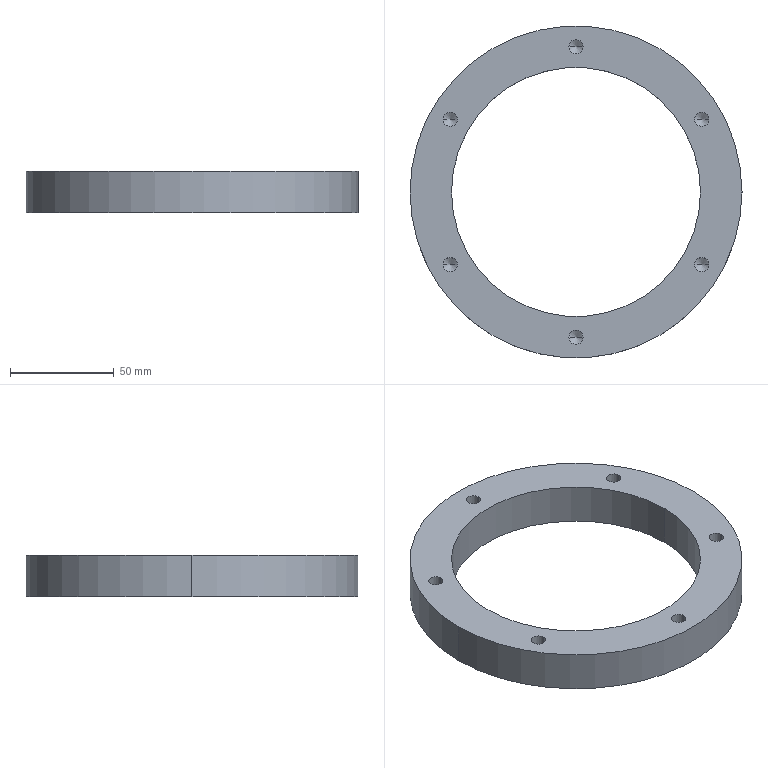Part | SolidWorks | features 3DProfileFeature 1, Extrusion 1, HoleWzd 1 | 1 solid | 30 faces | box 160 x 160 x 20 mm | volume 171859 mm3 | cylinder 16 | cone 12 | plane 2 | commonest cylinder face diameters 6.8 x12 120 x2 160 x2
STEP:
#1=CARTESIAN_POINT('',(-3.4,70.,2.));
#2=VERTEX_POINT('',#1);
#3=CARTESIAN_POINT('',(3.4,70.,2.));
#4=VERTEX_POINT('',#3);
#5=CARTESIAN_POINT('',(0.,70.,2.));
#6=DIRECTION('',(0.,0.,1.));
#7=DIRECTION('',(1.,0.,0.));
#8=AXIS2_PLACEMENT_3D('',#5,#6,#7);
#9=CIRCLE('',#8,3.4);
#10=EDGE_CURVE('',#2,#4,#9,.T.);
#11=ORIENTED_EDGE('',*,*,#10,.F.);
#12=CARTESIAN_POINT('',(-3.4,70.,20.));
#13=VERTEX_POINT('',#12);
#14=CARTESIAN_POINT('',(-3.4,70.,20.));
#15=DIRECTION('',(0.,0.,1.));
#16=VECTOR('',#15,1000.);
#17=LINE('',#14,#16);
#18=EDGE_CURVE('',#2,#13,#17,.T.);
#19=ORIENTED_EDGE('',*,*,#18,.T.);
#20=CARTESIAN_POINT('',(3.4,70.,20.));
#21=VERTEX_POINT('',#20);
#22=CARTESIAN_POINT('',(0.,70.,20.));
#23=DIRECTION('',(0.,0.,1.));
#24=DIRECTION('',(1.,0.,0.));
#25=AXIS2_PLACEMENT_3D('',#22,#23,#24);
#26=CIRCLE('',#25,3.4);
#27=EDGE_CURVE('',#13,#21,#26,.T.);
#28=ORIENTED_EDGE('',*,*,#27,.T.);
#29=CARTESIAN_POINT('',(3.4,70.,20.));
#30=DIRECTION('',(0.,0.,1.));
#31=VECTOR('',#30,1000.);
#32=LINE('',#29,#31);
#33=EDGE_CURVE('',#4,#21,#32,.T.);
#34=ORIENTED_EDGE('',*,*,#33,.F.);
#35=EDGE_LOOP('',(#11,#19,#28,#34));
#36=FACE_OUTER_BOUND('',#35,.T.);
#37=CARTESIAN_POINT('',(0.,70.,20.));
#38=DIRECTION('',(0.,0.,1.));
#39=DIRECTION('',(1.,0.,0.));
#40=AXIS2_PLACEMENT_3D('',#37,#38,#39);
#41=CYLINDRICAL_SURFACE('',#40,3.4);
#42=ADVANCED_FACE('',(#36),#41,.F.);
#43=CARTESIAN_POINT('',(-0.07144,70.,0.));
#44=VERTEX_POINT('',#43);
#45=CARTESIAN_POINT('',(0.07144,70.,0.));
#46=VERTEX_POINT('',#45);
#47=CARTESIAN_POINT('',(0.,70.,0.));
#48=DIRECTION('',(0.,0.,1.));
#49=DIRECTION('',(1.,0.,0.));
#50=AXIS2_PLACEMENT_3D('',#47,#48,#49);
#51=CIRCLE('',#50,0.07144);
#52=EDGE_CURVE('',#44,#46,#51,.T.);
#53=ORIENTED_EDGE('',*,*,#52,.F.);
#54=CARTESIAN_POINT('',(-3.4,70.,2.));
#55=DIRECTION('',(-0.8572,0.,0.515));
#56=VECTOR('',#55,1000.);
#57=LINE('',#54,#56);
#58=EDGE_CURVE('',#44,#2,#57,.T.);
#59=ORIENTED_EDGE('',*,*,#58,.T.);
#60=ORIENTED_EDGE('',*,*,#10,.T.);
#61=CARTESIAN_POINT('',(3.4,70.,2.));
#62=DIRECTION('',(0.8572,0.,0.515));
#63=VECTOR('',#62,1000.);
#64=LINE('',#61,#63);
#65=EDGE_CURVE('',#46,#4,#64,.T.);
#66=ORIENTED_EDGE('',*,*,#65,.F.);
#67=EDGE_LOOP('',(#53,#59,#60,#66));
#68=FACE_OUTER_BOUND('',#67,.T.);
#69=CARTESIAN_POINT('',(0.,70.,2.));
#70=DIRECTION('',(0.,0.,1.));
#71=DIRECTION('',(1.,0.,0.));
#72=AXIS2_PLACEMENT_3D('',#69,#70,#71);
#73=CONICAL_SURFACE('',#72,3.4,1.03);
#74=ADVANCED_FACE('',(#68),#73,.F.);
#75=CARTESIAN_POINT('',(57.222,35.,2.));
#76=VERTEX_POINT('',#75);
#77=CARTESIAN_POINT('',(64.022,35.,2.));
#78=VERTEX_POINT('',#77);
#79=CARTESIAN_POINT('',(60.622,35.,2.));
#80=DIRECTION('',(0.,0.,1.));
#81=DIRECTION('',(1.,0.,0.));
#82=AXIS2_PLACEMENT_3D('',#79,#80,#81);
#83=CIRCLE('',#82,3.4);
#84=EDGE_CURVE('',#76,#78,#83,.T.);
#85=ORIENTED_EDGE('',*,*,#84,.F.);
#86=CARTESIAN_POINT('',(57.222,35.,20.));
#87=VERTEX_POINT('',#86);
#88=CARTESIAN_POINT('',(57.222,35.,20.));
#89=DIRECTION('',(0.,0.,1.));
#90=VECTOR('',#89,1000.);
#91=LINE('',#88,#90);
#92=EDGE_CURVE('',#76,#87,#91,.T.);
#93=ORIENTED_EDGE('',*,*,#92,.T.);
#94=CARTESIAN_POINT('',(64.022,35.,20.));
#95=VERTEX_POINT('',#94);
#96=CARTESIAN_POINT('',(60.622,35.,20.));
#97=DIRECTION('',(0.,0.,1.));
#98=DIRECTION('',(1.,0.,0.));
#99=AXIS2_PLACEMENT_3D('',#96,#97,#98);
#100=CIRCLE('',#99,3.4);
#101=EDGE_CURVE('',#87,#95,#100,.T.);
#102=ORIENTED_EDGE('',*,*,#101,.T.);
#103=CARTESIAN_POINT('',(64.022,35.,20.));
#104=DIRECTION('',(0.,0.,1.));
#105=VECTOR('',#104,1000.);
#106=LINE('',#103,#105);
#107=EDGE_CURVE('',#78,#95,#106,.T.);
#108=ORIENTED_EDGE('',*,*,#107,.F.);
#109=EDGE_LOOP('',(#85,#93,#102,#108));
#110=FACE_OUTER_BOUND('',#109,.T.);
#111=CARTESIAN_POINT('',(60.622,35.,20.));
#112=DIRECTION('',(0.,0.,1.));
#113=DIRECTION('',(1.,0.,0.));
#114=AXIS2_PLACEMENT_3D('',#111,#112,#113);
#115=CYLINDRICAL_SURFACE('',#114,3.4);
#116=ADVANCED_FACE('',(#110),#115,.F.);
#117=CARTESIAN_POINT('',(60.55,35.,0.));
#118=VERTEX_POINT('',#117);
#119=CARTESIAN_POINT('',(60.693,35.,0.));
#120=VERTEX_POINT('',#119);
#121=CARTESIAN_POINT('',(60.622,35.,0.));
#122=DIRECTION('',(0.,0.,1.));
#123=DIRECTION('',(1.,0.,0.));
#124=AXIS2_PLACEMENT_3D('',#121,#122,#123);
#125=CIRCLE('',#124,0.07144);
#126=EDGE_CURVE('',#118,#120,#125,.T.);
#127=ORIENTED_EDGE('',*,*,#126,.F.);
#128=CARTESIAN_POINT('',(57.222,35.,2.));
#129=DIRECTION('',(-0.8572,0.,0.515));
#130=VECTOR('',#129,1000.);
#131=LINE('',#128,#130);
#132=EDGE_CURVE('',#118,#76,#131,.T.);
#133=ORIENTED_EDGE('',*,*,#132,.T.);
#134=ORIENTED_EDGE('',*,*,#84,.T.);
#135=CARTESIAN_POINT('',(64.022,35.,2.));
#136=DIRECTION('',(0.8572,0.,0.515));
#137=VECTOR('',#136,1000.);
#138=LINE('',#135,#137);
#139=EDGE_CURVE('',#120,#78,#138,.T.);
#140=ORIENTED_EDGE('',*,*,#139,.F.);
#141=EDGE_LOOP('',(#127,#133,#134,#140));
#142=FACE_OUTER_BOUND('',#141,.T.);
#143=CARTESIAN_POINT('',(60.622,35.,2.));
#144=DIRECTION('',(0.,0.,1.));
#145=DIRECTION('',(1.,0.,0.));
#146=AXIS2_PLACEMENT_3D('',#143,#144,#145);
#147=CONICAL_SURFACE('',#146,3.4,1.03);
#148=ADVANCED_FACE('',(#142),#147,.F.);
#149=CARTESIAN_POINT('',(57.222,-35.,2.));
#150=VERTEX_POINT('',#149);
#151=CARTESIAN_POINT('',(64.022,-35.,2.));
#152=VERTEX_POINT('',#151);
#153=CARTESIAN_POINT('',(60.622,-35.,2.));
#154=DIRECTION('',(0.,0.,1.));
#155=DIRECTION('',(1.,0.,0.));
#156=AXIS2_PLACEMENT_3D('',#153,#154,#155);
#157=CIRCLE('',#156,3.4);
#158=EDGE_CURVE('',#150,#152,#157,.T.);
#159=ORIENTED_EDGE('',*,*,#158,.F.);
#160=CARTESIAN_POINT('',(57.222,-35.,20.));
#161=VERTEX_POINT('',#160);
#162=CARTESIAN_POINT('',(57.222,-35.,20.));
#163=DIRECTION('',(0.,0.,1.));
#164=VECTOR('',#163,1000.);
#165=LINE('',#162,#164);
#166=EDGE_CURVE('',#150,#161,#165,.T.);
#167=ORIENTED_EDGE('',*,*,#166,.T.);
#168=CARTESIAN_POINT('',(64.022,-35.,20.));
#169=VERTEX_POINT('',#168);
#170=CARTESIAN_POINT('',(60.622,-35.,20.));
#171=DIRECTION('',(0.,0.,1.));
#172=DIRECTION('',(1.,0.,0.));
#173=AXIS2_PLACEMENT_3D('',#170,#171,#172);
#174=CIRCLE('',#173,3.4);
#175=EDGE_CURVE('',#161,#169,#174,.T.);
#176=ORIENTED_EDGE('',*,*,#175,.T.);
#177=CARTESIAN_POINT('',(64.022,-35.,20.));
#178=DIRECTION('',(0.,0.,1.));
#179=VECTOR('',#178,1000.);
#180=LINE('',#177,#179);
#181=EDGE_CURVE('',#152,#169,#180,.T.);
#182=ORIENTED_EDGE('',*,*,#181,.F.);
#183=EDGE_LOOP('',(#159,#167,#176,#182));
#184=FACE_OUTER_BOUND('',#183,.T.);
#185=CARTESIAN_POINT('',(60.622,-35.,20.));
#186=DIRECTION('',(0.,0.,1.));
#187=DIRECTION('',(1.,0.,0.));
#188=AXIS2_PLACEMENT_3D('',#185,#186,#187);
#189=CYLINDRICAL_SURFACE('',#188,3.4);
#190=ADVANCED_FACE('',(#184),#189,.F.);
#191=CARTESIAN_POINT('',(60.55,-35.,0.));
#192=VERTEX_POINT('',#191);
#193=CARTESIAN_POINT('',(60.693,-35.,0.));
#194=VERTEX_POINT('',#193);
#195=CARTESIAN_POINT('',(60.622,-35.,0.));
#196=DIRECTION('',(0.,0.,1.));
#197=DIRECTION('',(1.,0.,0.));
#198=AXIS2_PLACEMENT_3D('',#195,#196,#197);
#199=CIRCLE('',#198,0.07144);
#200=EDGE_CURVE('',#192,#194,#199,.T.);
#201=ORIENTED_EDGE('',*,*,#200,.F.);
#202=CARTESIAN_POINT('',(57.222,-35.,2.));
#203=DIRECTION('',(-0.8572,0.,0.515));
#204=VECTOR('',#203,1000.);
#205=LINE('',#202,#204);
#206=EDGE_CURVE('',#192,#150,#205,.T.);
#207=ORIENTED_EDGE('',*,*,#206,.T.);
#208=ORIENTED_EDGE('',*,*,#158,.T.);
#209=CARTESIAN_POINT('',(64.022,-35.,2.));
#210=DIRECTION('',(0.8572,0.,0.515));
#211=VECTOR('',#210,1000.);
#212=LINE('',#209,#211);
#213=EDGE_CURVE('',#194,#152,#212,.T.);
#214=ORIENTED_EDGE('',*,*,#213,.F.);
#215=EDGE_LOOP('',(#201,#207,#208,#214));
#216=FACE_OUTER_BOUND('',#215,.T.);
#217=CARTESIAN_POINT('',(60.622,-35.,2.));
#218=DIRECTION('',(0.,0.,1.));
#219=DIRECTION('',(1.,0.,0.));
#220=AXIS2_PLACEMENT_3D('',#217,#218,#219);
#221=CONICAL_SURFACE('',#220,3.4,1.03);
#222=ADVANCED_FACE('',(#216),#221,.F.);
#223=CARTESIAN_POINT('',(-3.4,-70.,2.));
#224=VERTEX_POINT('',#223);
#225=CARTESIAN_POINT('',(3.4,-70.,2.));
#226=VERTEX_POINT('',#225);
#227=CARTESIAN_POINT('',(0.,-70.,2.));
#228=DIRECTION('',(0.,0.,1.));
#229=DIRECTION('',(1.,0.,0.));
#230=AXIS2_PLACEMENT_3D('',#227,#228,#229);
#231=CIRCLE('',#230,3.4);
#232=EDGE_CURVE('',#224,#226,#231,.T.);
#233=ORIENTED_EDGE('',*,*,#232,.F.);
#234=CARTESIAN_POINT('',(-3.4,-70.,20.));
#235=VERTEX_POINT('',#234);
#236=CARTESIAN_POINT('',(-3.4,-70.,20.));
#237=DIRECTION('',(0.,0.,1.));
#238=VECTOR('',#237,1000.);
#239=LINE('',#236,#238);
#240=EDGE_CURVE('',#224,#235,#239,.T.);
#241=ORIENTED_EDGE('',*,*,#240,.T.);
#242=CARTESIAN_POINT('',(3.4,-70.,20.));
#243=VERTEX_POINT('',#242);
#244=CARTESIAN_POINT('',(0.,-70.,20.));
#245=DIRECTION('',(0.,0.,1.));
#246=DIRECTION('',(1.,0.,0.));
#247=AXIS2_PLACEMENT_3D('',#244,#245,#246);
#248=CIRCLE('',#247,3.4);
#249=EDGE_CURVE('',#235,#243,#248,.T.);
#250=ORIENTED_EDGE('',*,*,#249,.T.);
#251=CARTESIAN_POINT('',(3.4,-70.,20.));
#252=DIRECTION('',(0.,0.,1.));
#253=VECTOR('',#252,1000.);
#254=LINE('',#251,#253);
#255=EDGE_CURVE('',#226,#243,#254,.T.);
#256=ORIENTED_EDGE('',*,*,#255,.F.);
#257=EDGE_LOOP('',(#233,#241,#250,#256));
#258=FACE_OUTER_BOUND('',#257,.T.);
#259=CARTESIAN_POINT('',(0.,-70.,20.));
#260=DIRECTION('',(0.,0.,1.));
#261=DIRECTION('',(1.,0.,0.));
#262=AXIS2_PLACEMENT_3D('',#259,#260,#261);
#263=CYLINDRICAL_SURFACE('',#262,3.4);
#264=ADVANCED_FACE('',(#258),#263,.F.);
#265=CARTESIAN_POINT('',(-0.07144,-70.,0.));
#266=VERTEX_POINT('',#265);
#267=CARTESIAN_POINT('',(0.07144,-70.,0.));
#268=VERTEX_POINT('',#267);
#269=CARTESIAN_POINT('',(0.,-70.,0.));
#270=DIRECTION('',(0.,0.,1.));
#271=DIRECTION('',(1.,0.,0.));
#272=AXIS2_PLACEMENT_3D('',#269,#270,#271);
#273=CIRCLE('',#272,0.07144);
#274=EDGE_CURVE('',#266,#268,#273,.T.);
#275=ORIENTED_EDGE('',*,*,#274,.F.);
#276=CARTESIAN_POINT('',(-3.4,-70.,2.));
#277=DIRECTION('',(-0.8572,0.,0.515));
#278=VECTOR('',#277,1000.);
#279=LINE('',#276,#278);
#280=EDGE_CURVE('',#266,#224,#279,.T.);
#281=ORIENTED_EDGE('',*,*,#280,.T.);
#282=ORIENTED_EDGE('',*,*,#232,.T.);
#283=CARTESIAN_POINT('',(3.4,-70.,2.));
#284=DIRECTION('',(0.8572,0.,0.515));
#285=VECTOR('',#284,1000.);
#286=LINE('',#283,#285);
#287=EDGE_CURVE('',#268,#226,#286,.T.);
#288=ORIENTED_EDGE('',*,*,#287,.F.);
#289=EDGE_LOOP('',(#275,#281,#282,#288));
#290=FACE_OUTER_BOUND('',#289,.T.);
#291=CARTESIAN_POINT('',(0.,-70.,2.));
#292=DIRECTION('',(0.,0.,1.));
#293=DIRECTION('',(1.,0.,0.));
#294=AXIS2_PLACEMENT_3D('',#291,#292,#293);
#295=CONICAL_SURFACE('',#294,3.4,1.03);
#296=ADVANCED_FACE('',(#290),#295,.F.);
#297=CARTESIAN_POINT('',(-64.022,-35.,2.));
#298=VERTEX_POINT('',#297);
#299=CARTESIAN_POINT('',(-57.222,-35.,2.));
#300=VERTEX_POINT('',#299);
#301=CARTESIAN_POINT('',(-60.622,-35.,2.));
#302=DIRECTION('',(0.,0.,1.));
#303=DIRECTION('',(1.,0.,0.));
#304=AXIS2_PLACEMENT_3D('',#301,#302,#303);
#305=CIRCLE('',#304,3.4);
#306=EDGE_CURVE('',#298,#300,#305,.T.);
#307=ORIENTED_EDGE('',*,*,#306,.F.);
#308=CARTESIAN_POINT('',(-64.022,-35.,20.));
#309=VERTEX_POINT('',#308);
#310=CARTESIAN_POINT('',(-64.022,-35.,20.));
#311=DIRECTION('',(0.,0.,1.));
#312=VECTOR('',#311,1000.);
#313=LINE('',#310,#312);
#314=EDGE_CURVE('',#298,#309,#313,.T.);
#315=ORIENTED_EDGE('',*,*,#314,.T.);
#316=CARTESIAN_POINT('',(-57.222,-35.,20.));
#317=VERTEX_POINT('',#316);
#318=CARTESIAN_POINT('',(-60.622,-35.,20.));
#319=DIRECTION('',(0.,0.,1.));
#320=DIRECTION('',(1.,0.,0.));
#321=AXIS2_PLACEMENT_3D('',#318,#319,#320);
#322=CIRCLE('',#321,3.4);
#323=EDGE_CURVE('',#309,#317,#322,.T.);
#324=ORIENTED_EDGE('',*,*,#323,.T.);
#325=CARTESIAN_POINT('',(-57.222,-35.,20.));
#326=DIRECTION('',(0.,0.,1.));
#327=VECTOR('',#326,1000.);
#328=LINE('',#325,#327);
#329=EDGE_CURVE('',#300,#317,#328,.T.);
#330=ORIENTED_EDGE('',*,*,#329,.F.);
#331=EDGE_LOOP('',(#307,#315,#324,#330));
#332=FACE_OUTER_BOUND('',#331,.T.);
#333=CARTESIAN_POINT('',(-60.622,-35.,20.));
#334=DIRECTION('',(0.,0.,1.));
#335=DIRECTION('',(1.,0.,0.));
#336=AXIS2_PLACEMENT_3D('',#333,#334,#335);
#337=CYLINDRICAL_SURFACE('',#336,3.4);
#338=ADVANCED_FACE('',(#332),#337,.F.);
#339=CARTESIAN_POINT('',(-60.693,-35.,0.));
#340=VERTEX_POINT('',#339);
#341=CARTESIAN_POINT('',(-60.55,-35.,0.));
#342=VERTEX_POINT('',#341);
#343=CARTESIAN_POINT('',(-60.622,-35.,0.));
#344=DIRECTION('',(0.,0.,1.));
#345=DIRECTION('',(1.,0.,0.));
#346=AXIS2_PLACEMENT_3D('',#343,#344,#345);
#347=CIRCLE('',#346,0.07144);
#348=EDGE_CURVE('',#340,#342,#347,.T.);
#349=ORIENTED_EDGE('',*,*,#348,.F.);
#350=CARTESIAN_POINT('',(-64.022,-35.,2.));
#351=DIRECTION('',(-0.8572,0.,0.515));
#352=VECTOR('',#351,1000.);
#353=LINE('',#350,#352);
#354=EDGE_CURVE('',#340,#298,#353,.T.);
#355=ORIENTED_EDGE('',*,*,#354,.T.);
#356=ORIENTED_EDGE('',*,*,#306,.T.);
#357=CARTESIAN_POINT('',(-57.222,-35.,2.));
#358=DIRECTION('',(0.8572,0.,0.515));
#359=VECTOR('',#358,1000.);
#360=LINE('',#357,#359);
#361=EDGE_CURVE('',#342,#300,#360,.T.);
#362=ORIENTED_EDGE('',*,*,#361,.F.);
#363=EDGE_LOOP('',(#349,#355,#356,#362));
#364=FACE_OUTER_BOUND('',#363,.T.);
#365=CARTESIAN_POINT('',(-60.622,-35.,2.));
#366=DIRECTION('',(0.,0.,1.));
#367=DIRECTION('',(1.,0.,0.));
#368=AXIS2_PLACEMENT_3D('',#365,#366,#367);
#369=CONICAL_SURFACE('',#368,3.4,1.03);
#370=ADVANCED_FACE('',(#364),#369,.F.);
#371=CARTESIAN_POINT('',(-64.022,35.,2.));
#372=VERTEX_POINT('',#371);
#373=CARTESIAN_POINT('',(-57.222,35.,2.));
#374=VERTEX_POINT('',#373);
#375=CARTESIAN_POINT('',(-60.622,35.,2.));
#376=DIRECTION('',(0.,0.,1.));
#377=DIRECTION('',(1.,0.,0.));
#378=AXIS2_PLACEMENT_3D('',#375,#376,#377);
#379=CIRCLE('',#378,3.4);
#380=EDGE_CURVE('',#372,#374,#379,.T.);
#381=ORIENTED_EDGE('',*,*,#380,.F.);
#382=CARTESIAN_POINT('',(-64.022,35.,20.));
#383=VERTEX_POINT('',#382);
#384=CARTESIAN_POINT('',(-64.022,35.,20.));
#385=DIRECTION('',(0.,0.,1.));
#386=VECTOR('',#385,1000.);
#387=LINE('',#384,#386);
#388=EDGE_CURVE('',#372,#383,#387,.T.);
#389=ORIENTED_EDGE('',*,*,#388,.T.);
#390=CARTESIAN_POINT('',(-57.222,35.,20.));
#391=VERTEX_POINT('',#390);
#392=CARTESIAN_POINT('',(-60.622,35.,20.));
#393=DIRECTION('',(0.,0.,1.));
#394=DIRECTION('',(1.,0.,0.));
#395=AXIS2_PLACEMENT_3D('',#392,#393,#394);
#396=CIRCLE('',#395,3.4);
#397=EDGE_CURVE('',#383,#391,#396,.T.);
#398=ORIENTED_EDGE('',*,*,#397,.T.);
#399=CARTESIAN_POINT('',(-57.222,35.,20.));
#400=DIRECTION('',(0.,0.,1.));
#401=VECTOR('',#400,1000.);
#402=LINE('',#399,#401);
#403=EDGE_CURVE('',#374,#391,#402,.T.);
#404=ORIENTED_EDGE('',*,*,#403,.F.);
#405=EDGE_LOOP('',(#381,#389,#398,#404));
#406=FACE_OUTER_BOUND('',#405,.T.);
#407=CARTESIAN_POINT('',(-60.622,35.,20.));
#408=DIRECTION('',(0.,0.,1.));
#409=DIRECTION('',(1.,0.,0.));
#410=AXIS2_PLACEMENT_3D('',#407,#408,#409);
#411=CYLINDRICAL_SURFACE('',#410,3.4);
#412=ADVANCED_FACE('',(#406),#411,.F.);
#413=CARTESIAN_POINT('',(-60.693,35.,0.));
#414=VERTEX_POINT('',#413);
#415=CARTESIAN_POINT('',(-60.55,35.,0.));
#416=VERTEX_POINT('',#415);
#417=CARTESIAN_POINT('',(-60.622,35.,0.));
#418=DIRECTION('',(0.,0.,1.));
#419=DIRECTION('',(1.,0.,0.));
#420=AXIS2_PLACEMENT_3D('',#417,#418,#419);
#421=CIRCLE('',#420,0.07144);
#422=EDGE_CURVE('',#414,#416,#421,.T.);
#423=ORIENTED_EDGE('',*,*,#422,.F.);
#424=CARTESIAN_POINT('',(-64.022,35.,2.));
#425=DIRECTION('',(-0.8572,0.,0.515));
#426=VECTOR('',#425,1000.);
#427=LINE('',#424,#426);
#428=EDGE_CURVE('',#414,#372,#427,.T.);
#429=ORIENTED_EDGE('',*,*,#428,.T.);
#430=ORIENTED_EDGE('',*,*,#380,.T.);
#431=CARTESIAN_POINT('',(-57.222,35.,2.));
#432=DIRECTION('',(0.8572,0.,0.515));
#433=VECTOR('',#432,1000.);
#434=LINE('',#431,#433);
#435=EDGE_CURVE('',#416,#374,#434,.T.);
#436=ORIENTED_EDGE('',*,*,#435,.F.);
#437=EDGE_LOOP('',(#423,#429,#430,#436));
#438=FACE_OUTER_BOUND('',#437,.T.);
#439=CARTESIAN_POINT('',(-60.622,35.,2.));
#440=DIRECTION('',(0.,0.,1.));
#441=DIRECTION('',(1.,0.,0.));
#442=AXIS2_PLACEMENT_3D('',#439,#440,#441);
#443=CONICAL_SURFACE('',#442,3.4,1.03);
#444=ADVANCED_FACE('',(#438),#443,.F.);
#445=CARTESIAN_POINT('',(-60.,0.,20.));
#446=VERTEX_POINT('',#445);
#447=CARTESIAN_POINT('',(60.,0.,20.));
#448=VERTEX_POINT('',#447);
#449=CARTESIAN_POINT('',(0.,0.,20.));
#450=DIRECTION('',(0.,0.,1.));
#451=DIRECTION('',(1.,0.,0.));
#452=AXIS2_PLACEMENT_3D('',#449,#450,#451);
#453=CIRCLE('',#452,60.);
#454=EDGE_CURVE('',#446,#448,#453,.T.);
#455=ORIENTED_EDGE('',*,*,#454,.T.);
#456=CARTESIAN_POINT('',(60.,0.,0.));
#457=VERTEX_POINT('',#456);
#458=CARTESIAN_POINT('',(60.,0.,20.));
#459=DIRECTION('',(0.,0.,-1.));
#460=VECTOR('',#459,1000.);
#461=LINE('',#458,#460);
#462=EDGE_CURVE('',#448,#457,#461,.T.);
#463=ORIENTED_EDGE('',*,*,#462,.T.);
#464=CARTESIAN_POINT('',(-60.,0.,0.));
#465=VERTEX_POINT('',#464);
#466=CARTESIAN_POINT('',(0.,0.,0.));
#467=DIRECTION('',(0.,0.,1.));
#468=DIRECTION('',(1.,0.,0.));
#469=AXIS2_PLACEMENT_3D('',#466,#467,#468);
#470=CIRCLE('',#469,60.);
#471=EDGE_CURVE('',#465,#457,#470,.T.);
#472=ORIENTED_EDGE('',*,*,#471,.F.);
#473=CARTESIAN_POINT('',(-60.,0.,20.));
#474=DIRECTION('',(0.,0.,-1.));
#475=VECTOR('',#474,1000.);
#476=LINE('',#473,#475);
#477=EDGE_CURVE('',#446,#465,#476,.T.);
#478=ORIENTED_EDGE('',*,*,#477,.F.);
#479=EDGE_LOOP('',(#455,#463,#472,#478));
#480=FACE_OUTER_BOUND('',#479,.T.);
#481=CARTESIAN_POINT('',(0.,0.,20.));
#482=DIRECTION('',(0.,0.,-1.));
#483=DIRECTION('',(-1.,0.,0.));
#484=AXIS2_PLACEMENT_3D('',#481,#482,#483);
#485=CYLINDRICAL_SURFACE('',#484,60.);
#486=ADVANCED_FACE('',(#480),#485,.F.);
#487=CARTESIAN_POINT('',(80.,0.,20.));
#488=VERTEX_POINT('',#487);
#489=CARTESIAN_POINT('',(-80.,0.,20.));
#490=VERTEX_POINT('',#489);
#491=CARTESIAN_POINT('',(0.,0.,20.));
#492=DIRECTION('',(0.,0.,1.));
#493=DIRECTION('',(1.,0.,0.));
#494=AXIS2_PLACEMENT_3D('',#491,#492,#493);
#495=CIRCLE('',#494,80.);
#496=EDGE_CURVE('',#488,#490,#495,.T.);
#497=ORIENTED_EDGE('',*,*,#496,.F.);
#498=CARTESIAN_POINT('',(80.,0.,0.));
#499=VERTEX_POINT('',#498);
#500=CARTESIAN_POINT('',(80.,0.,20.));
#501=DIRECTION('',(0.,0.,-1.));
#502=VECTOR('',#501,1000.);
#503=LINE('',#500,#502);
#504=EDGE_CURVE('',#488,#499,#503,.T.);
#505=ORIENTED_EDGE('',*,*,#504,.T.);
#506=CARTESIAN_POINT('',(-80.,0.,0.));
#507=VERTEX_POINT('',#506);
#508=CARTESIAN_POINT('',(0.,0.,0.));
#509=DIRECTION('',(0.,0.,1.));
#510=DIRECTION('',(1.,0.,0.));
#511=AXIS2_PLACEMENT_3D('',#508,#509,#510);
#512=CIRCLE('',#511,80.);
#513=EDGE_CURVE('',#499,#507,#512,.T.);
#514=ORIENTED_EDGE('',*,*,#513,.T.);
#515=CARTESIAN_POINT('',(-80.,0.,20.));
#516=DIRECTION('',(0.,0.,-1.));
#517=VECTOR('',#516,1000.);
#518=LINE('',#515,#517);
#519=EDGE_CURVE('',#490,#507,#518,.T.);
#520=ORIENTED_EDGE('',*,*,#519,.F.);
#521=EDGE_LOOP('',(#497,#505,#514,#520));
#522=FACE_OUTER_BOUND('',#521,.T.);
#523=CARTESIAN_POINT('',(0.,0.,20.));
#524=DIRECTION('',(0.,0.,-1.));
#525=DIRECTION('',(-1.,0.,0.));
#526=AXIS2_PLACEMENT_3D('',#523,#524,#525);
#527=CYLINDRICAL_SURFACE('',#526,80.);
#528=ADVANCED_FACE('',(#522),#527,.T.);
#529=CARTESIAN_POINT('',(0.,70.,20.));
#530=DIRECTION('',(0.,0.,1.));
#531=DIRECTION('',(1.,0.,0.));
#532=AXIS2_PLACEMENT_3D('',#529,#530,#531);
#533=CIRCLE('',#532,3.4);
#534=EDGE_CURVE('',#21,#13,#533,.T.);
#535=ORIENTED_EDGE('',*,*,#534,.F.);
#536=ORIENTED_EDGE('',*,*,#27,.F.);
#537=EDGE_LOOP('',(#535,#536));
#538=FACE_BOUND('',#537,.T.);
#539=CARTESIAN_POINT('',(60.622,35.,20.));
#540=DIRECTION('',(0.,0.,1.));
#541=DIRECTION('',(1.,0.,0.));
#542=AXIS2_PLACEMENT_3D('',#539,#540,#541);
#543=CIRCLE('',#542,3.4);
#544=EDGE_CURVE('',#95,#87,#543,.T.);
#545=ORIENTED_EDGE('',*,*,#544,.F.);
#546=ORIENTED_EDGE('',*,*,#101,.F.);
#547=EDGE_LOOP('',(#545,#546));
#548=FACE_BOUND('',#547,.T.);
#549=CARTESIAN_POINT('',(60.622,-35.,20.));
#550=DIRECTION('',(0.,0.,1.));
#551=DIRECTION('',(1.,0.,0.));
#552=AXIS2_PLACEMENT_3D('',#549,#550,#551);
#553=CIRCLE('',#552,3.4);
#554=EDGE_CURVE('',#169,#161,#553,.T.);
#555=ORIENTED_EDGE('',*,*,#554,.F.);
#556=ORIENTED_EDGE('',*,*,#175,.F.);
#557=EDGE_LOOP('',(#555,#556));
#558=FACE_BOUND('',#557,.T.);
#559=CARTESIAN_POINT('',(0.,-70.,20.));
#560=DIRECTION('',(0.,0.,1.));
#561=DIRECTION('',(1.,0.,0.));
#562=AXIS2_PLACEMENT_3D('',#559,#560,#561);
#563=CIRCLE('',#562,3.4);
#564=EDGE_CURVE('',#243,#235,#563,.T.);
#565=ORIENTED_EDGE('',*,*,#564,.F.);
#566=ORIENTED_EDGE('',*,*,#249,.F.);
#567=EDGE_LOOP('',(#565,#566));
#568=FACE_BOUND('',#567,.T.);
#569=CARTESIAN_POINT('',(-60.622,-35.,20.));
#570=DIRECTION('',(0.,0.,1.));
#571=DIRECTION('',(1.,0.,0.));
#572=AXIS2_PLACEMENT_3D('',#569,#570,#571);
#573=CIRCLE('',#572,3.4);
#574=EDGE_CURVE('',#317,#309,#573,.T.);
#575=ORIENTED_EDGE('',*,*,#574,.F.);
#576=ORIENTED_EDGE('',*,*,#323,.F.);
#577=EDGE_LOOP('',(#575,#576));
#578=FACE_BOUND('',#577,.T.);
#579=CARTESIAN_POINT('',(-60.622,35.,20.));
#580=DIRECTION('',(0.,0.,1.));
#581=DIRECTION('',(1.,0.,0.));
#582=AXIS2_PLACEMENT_3D('',#579,#580,#581);
#583=CIRCLE('',#582,3.4);
#584=EDGE_CURVE('',#391,#383,#583,.T.);
#585=ORIENTED_EDGE('',*,*,#584,.F.);
#586=ORIENTED_EDGE('',*,*,#397,.F.);
#587=EDGE_LOOP('',(#585,#586));
#588=FACE_BOUND('',#587,.T.);
#589=CARTESIAN_POINT('',(0.,0.,20.));
#590=DIRECTION('',(0.,0.,1.));
#591=DIRECTION('',(1.,0.,0.));
#592=AXIS2_PLACEMENT_3D('',#589,#590,#591);
#593=CIRCLE('',#592,80.);
#594=EDGE_CURVE('',#490,#488,#593,.T.);
#595=ORIENTED_EDGE('',*,*,#594,.T.);
#596=ORIENTED_EDGE('',*,*,#496,.T.);
#597=EDGE_LOOP('',(#595,#596));
#598=FACE_OUTER_BOUND('',#597,.T.);
#599=ORIENTED_EDGE('',*,*,#454,.F.);
#600=CARTESIAN_POINT('',(0.,0.,20.));
#601=DIRECTION('',(0.,0.,1.));
#602=DIRECTION('',(1.,0.,0.));
#603=AXIS2_PLACEMENT_3D('',#600,#601,#602);
#604=CIRCLE('',#603,60.);
#605=EDGE_CURVE('',#448,#446,#604,.T.);
#606=ORIENTED_EDGE('',*,*,#605,.F.);
#607=EDGE_LOOP('',(#599,#606));
#608=FACE_BOUND('',#607,.T.);
#609=CARTESIAN_POINT('',(0.,0.,20.));
#610=DIRECTION('',(0.,0.,1.));
#611=DIRECTION('',(1.,0.,0.));
#612=AXIS2_PLACEMENT_3D('',#609,#610,#611);
#613=PLANE('',#612);
#614=ADVANCED_FACE('',(#538,#548,#558,#568,#578,#588,#598,#608),#613,.T.);
#615=CARTESIAN_POINT('',(0.,70.,0.));
#616=DIRECTION('',(0.,0.,1.));
#617=DIRECTION('',(1.,0.,0.));
#618=AXIS2_PLACEMENT_3D('',#615,#616,#617);
#619=CIRCLE('',#618,0.07144);
#620=EDGE_CURVE('',#46,#44,#619,.T.);
#621=ORIENTED_EDGE('',*,*,#620,.T.);
#622=ORIENTED_EDGE('',*,*,#52,.T.);
#623=EDGE_LOOP('',(#621,#622));
#624=FACE_BOUND('',#623,.T.);
#625=CARTESIAN_POINT('',(60.622,35.,0.));
#626=DIRECTION('',(0.,0.,1.));
#627=DIRECTION('',(1.,0.,0.));
#628=AXIS2_PLACEMENT_3D('',#625,#626,#627);
#629=CIRCLE('',#628,0.07144);
#630=EDGE_CURVE('',#120,#118,#629,.T.);
#631=ORIENTED_EDGE('',*,*,#630,.T.);
#632=ORIENTED_EDGE('',*,*,#126,.T.);
#633=EDGE_LOOP('',(#631,#632));
#634=FACE_BOUND('',#633,.T.);
#635=CARTESIAN_POINT('',(60.622,-35.,0.));
#636=DIRECTION('',(0.,0.,1.));
#637=DIRECTION('',(1.,0.,0.));
#638=AXIS2_PLACEMENT_3D('',#635,#636,#637);
#639=CIRCLE('',#638,0.07144);
#640=EDGE_CURVE('',#194,#192,#639,.T.);
#641=ORIENTED_EDGE('',*,*,#640,.T.);
#642=ORIENTED_EDGE('',*,*,#200,.T.);
#643=EDGE_LOOP('',(#641,#642));
#644=FACE_BOUND('',#643,.T.);
#645=CARTESIAN_POINT('',(0.,-70.,0.));
#646=DIRECTION('',(0.,0.,1.));
#647=DIRECTION('',(1.,0.,0.));
#648=AXIS2_PLACEMENT_3D('',#645,#646,#647);
#649=CIRCLE('',#648,0.07144);
#650=EDGE_CURVE('',#268,#266,#649,.T.);
#651=ORIENTED_EDGE('',*,*,#650,.T.);
#652=ORIENTED_EDGE('',*,*,#274,.T.);
#653=EDGE_LOOP('',(#651,#652));
#654=FACE_BOUND('',#653,.T.);
#655=CARTESIAN_POINT('',(-60.622,-35.,0.));
#656=DIRECTION('',(0.,0.,1.));
#657=DIRECTION('',(1.,0.,0.));
#658=AXIS2_PLACEMENT_3D('',#655,#656,#657);
#659=CIRCLE('',#658,0.07144);
#660=EDGE_CURVE('',#342,#340,#659,.T.);
#661=ORIENTED_EDGE('',*,*,#660,.T.);
#662=ORIENTED_EDGE('',*,*,#348,.T.);
#663=EDGE_LOOP('',(#661,#662));
#664=FACE_BOUND('',#663,.T.);
#665=CARTESIAN_POINT('',(-60.622,35.,0.));
#666=DIRECTION('',(0.,0.,1.));
#667=DIRECTION('',(1.,0.,0.));
#668=AXIS2_PLACEMENT_3D('',#665,#666,#667);
#669=CIRCLE('',#668,0.07144);
#670=EDGE_CURVE('',#416,#414,#669,.T.);
#671=ORIENTED_EDGE('',*,*,#670,.T.);
#672=ORIENTED_EDGE('',*,*,#422,.T.);
#673=EDGE_LOOP('',(#671,#672));
#674=FACE_BOUND('',#673,.T.);
#675=CARTESIAN_POINT('',(0.,0.,0.));
#676=DIRECTION('',(0.,0.,1.));
#677=DIRECTION('',(1.,0.,0.));
#678=AXIS2_PLACEMENT_3D('',#675,#676,#677);
#679=CIRCLE('',#678,80.);
#680=EDGE_CURVE('',#507,#499,#679,.T.);
#681=ORIENTED_EDGE('',*,*,#680,.F.);
#682=ORIENTED_EDGE('',*,*,#513,.F.);
#683=EDGE_LOOP('',(#681,#682));
#684=FACE_OUTER_BOUND('',#683,.T.);
#685=ORIENTED_EDGE('',*,*,#471,.T.);
#686=CARTESIAN_POINT('',(0.,0.,0.));
#687=DIRECTION('',(0.,0.,1.));
#688=DIRECTION('',(1.,0.,0.));
#689=AXIS2_PLACEMENT_3D('',#686,#687,#688);
#690=CIRCLE('',#689,60.);
#691=EDGE_CURVE('',#457,#465,#690,.T.);
#692=ORIENTED_EDGE('',*,*,#691,.T.);
#693=EDGE_LOOP('',(#685,#692));
#694=FACE_BOUND('',#693,.T.);
#695=CARTESIAN_POINT('',(0.,0.,0.));
#696=DIRECTION('',(0.,0.,1.));
#697=DIRECTION('',(1.,0.,0.));
#698=AXIS2_PLACEMENT_3D('',#695,#696,#697);
#699=PLANE('',#698);
#700=ADVANCED_FACE('',(#624,#634,#644,#654,#664,#674,#684,#694),#699,.F.);
#701=ORIENTED_EDGE('',*,*,#504,.F.);
#702=ORIENTED_EDGE('',*,*,#594,.F.);
#703=ORIENTED_EDGE('',*,*,#519,.T.);
#704=ORIENTED_EDGE('',*,*,#680,.T.);
#705=EDGE_LOOP('',(#701,#702,#703,#704));
#706=FACE_OUTER_BOUND('',#705,.T.);
#707=CARTESIAN_POINT('',(0.,0.,20.));
#708=DIRECTION('',(0.,0.,-1.));
#709=DIRECTION('',(-1.,0.,0.));
#710=AXIS2_PLACEMENT_3D('',#707,#708,#709);
#711=CYLINDRICAL_SURFACE('',#710,80.);
#712=ADVANCED_FACE('',(#706),#711,.T.);
#713=ORIENTED_EDGE('',*,*,#462,.F.);
#714=ORIENTED_EDGE('',*,*,#605,.T.);
#715=ORIENTED_EDGE('',*,*,#477,.T.);
#716=ORIENTED_EDGE('',*,*,#691,.F.);
#717=EDGE_LOOP('',(#713,#714,#715,#716));
#718=FACE_OUTER_BOUND('',#717,.T.);
#719=CARTESIAN_POINT('',(0.,0.,20.));
#720=DIRECTION('',(0.,0.,-1.));
#721=DIRECTION('',(-1.,0.,0.));
#722=AXIS2_PLACEMENT_3D('',#719,#720,#721);
#723=CYLINDRICAL_SURFACE('',#722,60.);
#724=ADVANCED_FACE('',(#718),#723,.F.);
#725=ORIENTED_EDGE('',*,*,#428,.F.);
#726=ORIENTED_EDGE('',*,*,#670,.F.);
#727=ORIENTED_EDGE('',*,*,#435,.T.);
#728=CARTESIAN_POINT('',(-60.622,35.,2.));
#729=DIRECTION('',(0.,0.,1.));
#730=DIRECTION('',(1.,0.,0.));
#731=AXIS2_PLACEMENT_3D('',#728,#729,#730);
#732=CIRCLE('',#731,3.4);
#733=EDGE_CURVE('',#374,#372,#732,.T.);
#734=ORIENTED_EDGE('',*,*,#733,.T.);
#735=EDGE_LOOP('',(#725,#726,#727,#734));
#736=FACE_OUTER_BOUND('',#735,.T.);
#737=CARTESIAN_POINT('',(-60.622,35.,2.));
#738=DIRECTION('',(0.,0.,1.));
#739=DIRECTION('',(1.,0.,0.));
#740=AXIS2_PLACEMENT_3D('',#737,#738,#739);
#741=CONICAL_SURFACE('',#740,3.4,1.03);
#742=ADVANCED_FACE('',(#736),#741,.F.);
#743=ORIENTED_EDGE('',*,*,#388,.F.);
#744=ORIENTED_EDGE('',*,*,#733,.F.);
#745=ORIENTED_EDGE('',*,*,#403,.T.);
#746=ORIENTED_EDGE('',*,*,#584,.T.);
#747=EDGE_LOOP('',(#743,#744,#745,#746));
#748=FACE_OUTER_BOUND('',#747,.T.);
#749=CARTESIAN_POINT('',(-60.622,35.,20.));
#750=DIRECTION('',(0.,0.,1.));
#751=DIRECTION('',(1.,0.,0.));
#752=AXIS2_PLACEMENT_3D('',#749,#750,#751);
#753=CYLINDRICAL_SURFACE('',#752,3.4);
#754=ADVANCED_FACE('',(#748),#753,.F.);
#755=ORIENTED_EDGE('',*,*,#354,.F.);
#756=ORIENTED_EDGE('',*,*,#660,.F.);
#757=ORIENTED_EDGE('',*,*,#361,.T.);
#758=CARTESIAN_POINT('',(-60.622,-35.,2.));
#759=DIRECTION('',(0.,0.,1.));
#760=DIRECTION('',(1.,0.,0.));
#761=AXIS2_PLACEMENT_3D('',#758,#759,#760);
#762=CIRCLE('',#761,3.4);
#763=EDGE_CURVE('',#300,#298,#762,.T.);
#764=ORIENTED_EDGE('',*,*,#763,.T.);
#765=EDGE_LOOP('',(#755,#756,#757,#764));
#766=FACE_OUTER_BOUND('',#765,.T.);
#767=CARTESIAN_POINT('',(-60.622,-35.,2.));
#768=DIRECTION('',(0.,0.,1.));
#769=DIRECTION('',(1.,0.,0.));
#770=AXIS2_PLACEMENT_3D('',#767,#768,#769);
#771=CONICAL_SURFACE('',#770,3.4,1.03);
#772=ADVANCED_FACE('',(#766),#771,.F.);
#773=ORIENTED_EDGE('',*,*,#314,.F.);
#774=ORIENTED_EDGE('',*,*,#763,.F.);
#775=ORIENTED_EDGE('',*,*,#329,.T.);
#776=ORIENTED_EDGE('',*,*,#574,.T.);
#777=EDGE_LOOP('',(#773,#774,#775,#776));
#778=FACE_OUTER_BOUND('',#777,.T.);
#779=CARTESIAN_POINT('',(-60.622,-35.,20.));
#780=DIRECTION('',(0.,0.,1.));
#781=DIRECTION('',(1.,0.,0.));
#782=AXIS2_PLACEMENT_3D('',#779,#780,#781);
#783=CYLINDRICAL_SURFACE('',#782,3.4);
#784=ADVANCED_FACE('',(#778),#783,.F.);
#785=ORIENTED_EDGE('',*,*,#280,.F.);
#786=ORIENTED_EDGE('',*,*,#650,.F.);
#787=ORIENTED_EDGE('',*,*,#287,.T.);
#788=CARTESIAN_POINT('',(0.,-70.,2.));
#789=DIRECTION('',(0.,0.,1.));
#790=DIRECTION('',(1.,0.,0.));
#791=AXIS2_PLACEMENT_3D('',#788,#789,#790);
#792=CIRCLE('',#791,3.4);
#793=EDGE_CURVE('',#226,#224,#792,.T.);
#794=ORIENTED_EDGE('',*,*,#793,.T.);
#795=EDGE_LOOP('',(#785,#786,#787,#794));
#796=FACE_OUTER_BOUND('',#795,.T.);
#797=CARTESIAN_POINT('',(0.,-70.,2.));
#798=DIRECTION('',(0.,0.,1.));
#799=DIRECTION('',(1.,0.,0.));
#800=AXIS2_PLACEMENT_3D('',#797,#798,#799);
#801=CONICAL_SURFACE('',#800,3.4,1.03);
#802=ADVANCED_FACE('',(#796),#801,.F.);
#803=ORIENTED_EDGE('',*,*,#240,.F.);
#804=ORIENTED_EDGE('',*,*,#793,.F.);
#805=ORIENTED_EDGE('',*,*,#255,.T.);
#806=ORIENTED_EDGE('',*,*,#564,.T.);
#807=EDGE_LOOP('',(#803,#804,#805,#806));
#808=FACE_OUTER_BOUND('',#807,.T.);
#809=CARTESIAN_POINT('',(0.,-70.,20.));
#810=DIRECTION('',(0.,0.,1.));
#811=DIRECTION('',(1.,0.,0.));
#812=AXIS2_PLACEMENT_3D('',#809,#810,#811);
#813=CYLINDRICAL_SURFACE('',#812,3.4);
#814=ADVANCED_FACE('',(#808),#813,.F.);
#815=ORIENTED_EDGE('',*,*,#206,.F.);
#816=ORIENTED_EDGE('',*,*,#640,.F.);
#817=ORIENTED_EDGE('',*,*,#213,.T.);
#818=CARTESIAN_POINT('',(60.622,-35.,2.));
#819=DIRECTION('',(0.,0.,1.));
#820=DIRECTION('',(1.,0.,0.));
#821=AXIS2_PLACEMENT_3D('',#818,#819,#820);
#822=CIRCLE('',#821,3.4);
#823=EDGE_CURVE('',#152,#150,#822,.T.);
#824=ORIENTED_EDGE('',*,*,#823,.T.);
#825=EDGE_LOOP('',(#815,#816,#817,#824));
#826=FACE_OUTER_BOUND('',#825,.T.);
#827=CARTESIAN_POINT('',(60.622,-35.,2.));
#828=DIRECTION('',(0.,0.,1.));
#829=DIRECTION('',(1.,0.,0.));
#830=AXIS2_PLACEMENT_3D('',#827,#828,#829);
#831=CONICAL_SURFACE('',#830,3.4,1.03);
#832=ADVANCED_FACE('',(#826),#831,.F.);
#833=ORIENTED_EDGE('',*,*,#166,.F.);
#834=ORIENTED_EDGE('',*,*,#823,.F.);
#835=ORIENTED_EDGE('',*,*,#181,.T.);
#836=ORIENTED_EDGE('',*,*,#554,.T.);
#837=EDGE_LOOP('',(#833,#834,#835,#836));
#838=FACE_OUTER_BOUND('',#837,.T.);
#839=CARTESIAN_POINT('',(60.622,-35.,20.));
#840=DIRECTION('',(0.,0.,1.));
#841=DIRECTION('',(1.,0.,0.));
#842=AXIS2_PLACEMENT_3D('',#839,#840,#841);
#843=CYLINDRICAL_SURFACE('',#842,3.4);
#844=ADVANCED_FACE('',(#838),#843,.F.);
#845=ORIENTED_EDGE('',*,*,#132,.F.);
#846=ORIENTED_EDGE('',*,*,#630,.F.);
#847=ORIENTED_EDGE('',*,*,#139,.T.);
#848=CARTESIAN_POINT('',(60.622,35.,2.));
#849=DIRECTION('',(0.,0.,1.));
#850=DIRECTION('',(1.,0.,0.));
#851=AXIS2_PLACEMENT_3D('',#848,#849,#850);
#852=CIRCLE('',#851,3.4);
#853=EDGE_CURVE('',#78,#76,#852,.T.);
#854=ORIENTED_EDGE('',*,*,#853,.T.);
#855=EDGE_LOOP('',(#845,#846,#847,#854));
#856=FACE_OUTER_BOUND('',#855,.T.);
#857=CARTESIAN_POINT('',(60.622,35.,2.));
#858=DIRECTION('',(0.,0.,1.));
#859=DIRECTION('',(1.,0.,0.));
#860=AXIS2_PLACEMENT_3D('',#857,#858,#859);
#861=CONICAL_SURFACE('',#860,3.4,1.03);
#862=ADVANCED_FACE('',(#856),#861,.F.);
#863=ORIENTED_EDGE('',*,*,#92,.F.);
#864=ORIENTED_EDGE('',*,*,#853,.F.);
#865=ORIENTED_EDGE('',*,*,#107,.T.);
#866=ORIENTED_EDGE('',*,*,#544,.T.);
#867=EDGE_LOOP('',(#863,#864,#865,#866));
#868=FACE_OUTER_BOUND('',#867,.T.);
#869=CARTESIAN_POINT('',(60.622,35.,20.));
#870=DIRECTION('',(0.,0.,1.));
#871=DIRECTION('',(1.,0.,0.));
#872=AXIS2_PLACEMENT_3D('',#869,#870,#871);
#873=CYLINDRICAL_SURFACE('',#872,3.4);
#874=ADVANCED_FACE('',(#868),#873,.F.);
#875=ORIENTED_EDGE('',*,*,#58,.F.);
#876=ORIENTED_EDGE('',*,*,#620,.F.);
#877=ORIENTED_EDGE('',*,*,#65,.T.);
#878=CARTESIAN_POINT('',(0.,70.,2.));
#879=DIRECTION('',(0.,0.,1.));
#880=DIRECTION('',(1.,0.,0.));
#881=AXIS2_PLACEMENT_3D('',#878,#879,#880);
#882=CIRCLE('',#881,3.4);
#883=EDGE_CURVE('',#4,#2,#882,.T.);
#884=ORIENTED_EDGE('',*,*,#883,.T.);
#885=EDGE_LOOP('',(#875,#876,#877,#884));
#886=FACE_OUTER_BOUND('',#885,.T.);
#887=CARTESIAN_POINT('',(0.,70.,2.));
#888=DIRECTION('',(0.,0.,1.));
#889=DIRECTION('',(1.,0.,0.));
#890=AXIS2_PLACEMENT_3D('',#887,#888,#889);
#891=CONICAL_SURFACE('',#890,3.4,1.03);
#892=ADVANCED_FACE('',(#886),#891,.F.);
#893=ORIENTED_EDGE('',*,*,#18,.F.);
#894=ORIENTED_EDGE('',*,*,#883,.F.);
#895=ORIENTED_EDGE('',*,*,#33,.T.);
#896=ORIENTED_EDGE('',*,*,#534,.T.);
#897=EDGE_LOOP('',(#893,#894,#895,#896));
#898=FACE_OUTER_BOUND('',#897,.T.);
#899=CARTESIAN_POINT('',(0.,70.,20.));
#900=DIRECTION('',(0.,0.,1.));
#901=DIRECTION('',(1.,0.,0.));
#902=AXIS2_PLACEMENT_3D('',#899,#900,#901);
#903=CYLINDRICAL_SURFACE('',#902,3.4);
#904=ADVANCED_FACE('',(#898),#903,.F.);
#905=CLOSED_SHELL('',(#42,#74,#116,#148,#190,#222,#264,#296,#338,#370,#412,#444,#486,#528,#614,#700,#712,#724,#742,#754,#772,#784,#802,#814,#832,#844,#862,#874,#892,#904));
#906=MANIFOLD_SOLID_BREP('',#905);
#907=CARTESIAN_POINT('',(0.,0.,0.));
#908=DIRECTION('',(0.,0.,1.));
#909=DIRECTION('',(1.,0.,0.));
#910=AXIS2_PLACEMENT_3D('',#907,#908,#909);
#911=(LENGTH_UNIT()NAMED_UNIT(*)SI_UNIT(.MILLI.,.METRE.));
#912=UNCERTAINTY_MEASURE_WITH_UNIT(LENGTH_MEASURE(0.00001),#911,'','');
#913=(NAMED_UNIT(*)PLANE_ANGLE_UNIT()SI_UNIT($,.RADIAN.));
#914=(NAMED_UNIT(*)SI_UNIT($,.STERADIAN.)SOLID_ANGLE_UNIT());
#915=(GEOMETRIC_REPRESENTATION_CONTEXT(3)GLOBAL_UNCERTAINTY_ASSIGNED_CONTEXT((#912))GLOBAL_UNIT_ASSIGNED_CONTEXT((#911,#913,#914))REPRESENTATION_CONTEXT('',''));
#916=ADVANCED_BREP_SHAPE_REPRESENTATION('',(#906,#910),#915);